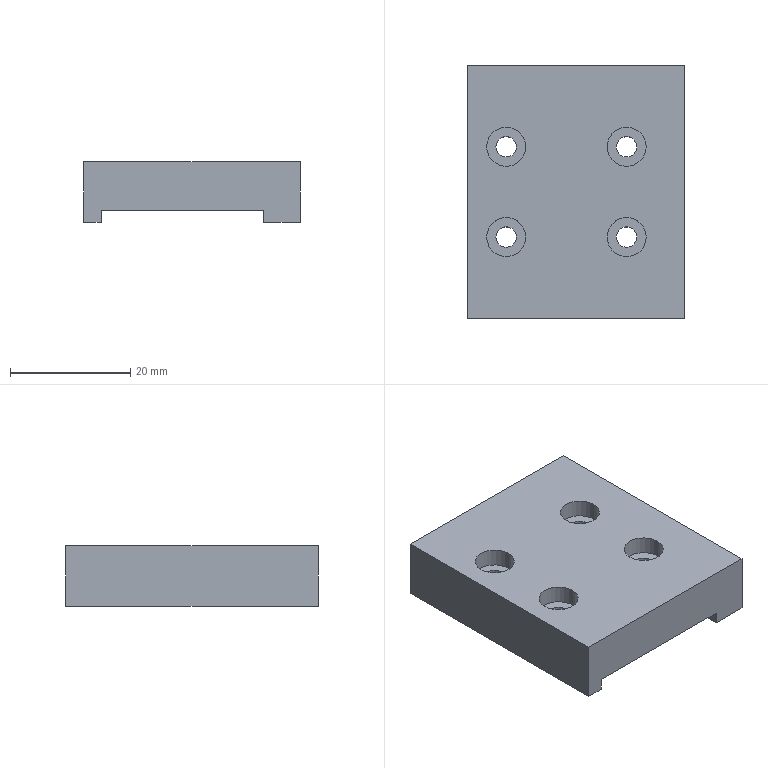Part | NX | features BREP 1 | 1 solid | 30 faces | box 36 x 42 x 10 mm | volume 12272 mm3 | cylinder 16 | plane 14 | commonest cylinder face diameters 3.4 x8 6.5 x8
STEP:
#1=CARTESIAN_POINT('',(-13.25,63.775,7.));
#2=VERTEX_POINT('',#1);
#3=CARTESIAN_POINT('',(-6.75,63.775,7.));
#4=VERTEX_POINT('',#3);
#5=CARTESIAN_POINT('',(-10.,63.775,7.));
#6=DIRECTION('',(0.,0.,1.));
#7=DIRECTION('',(1.,0.,0.));
#8=AXIS2_PLACEMENT_3D('',#5,#6,#7);
#9=CIRCLE('',#8,3.25);
#10=EDGE_CURVE('',#2,#4,#9,.T.);
#11=ORIENTED_EDGE('',*,*,#10,.F.);
#12=CARTESIAN_POINT('',(-13.25,63.775,10.));
#13=VERTEX_POINT('',#12);
#14=CARTESIAN_POINT('',(-13.25,63.775,10.));
#15=DIRECTION('',(0.,0.,1.));
#16=VECTOR('',#15,1000.);
#17=LINE('',#14,#16);
#18=EDGE_CURVE('',#13,#2,#17,.F.);
#19=ORIENTED_EDGE('',*,*,#18,.F.);
#20=CARTESIAN_POINT('',(-6.75,63.775,10.));
#21=VERTEX_POINT('',#20);
#22=CARTESIAN_POINT('',(-10.,63.775,10.));
#23=DIRECTION('',(0.,0.,1.));
#24=DIRECTION('',(1.,0.,0.));
#25=AXIS2_PLACEMENT_3D('',#22,#23,#24);
#26=CIRCLE('',#25,3.25);
#27=EDGE_CURVE('',#13,#21,#26,.T.);
#28=ORIENTED_EDGE('',*,*,#27,.T.);
#29=CARTESIAN_POINT('',(-6.75,63.775,10.));
#30=DIRECTION('',(0.,0.,1.));
#31=VECTOR('',#30,1000.);
#32=LINE('',#29,#31);
#33=EDGE_CURVE('',#21,#4,#32,.F.);
#34=ORIENTED_EDGE('',*,*,#33,.T.);
#35=EDGE_LOOP('',(#11,#19,#28,#34));
#36=FACE_BOUND('',#35,.T.);
#37=CARTESIAN_POINT('',(-10.,63.775,10.));
#38=DIRECTION('',(0.,0.,1.));
#39=DIRECTION('',(1.,0.,0.));
#40=AXIS2_PLACEMENT_3D('',#37,#38,#39);
#41=CYLINDRICAL_SURFACE('',#40,3.25);
#42=ADVANCED_FACE('',(#36),#41,.F.);
#43=CARTESIAN_POINT('',(-11.7,63.775,2.));
#44=VERTEX_POINT('',#43);
#45=CARTESIAN_POINT('',(-8.3,63.775,2.));
#46=VERTEX_POINT('',#45);
#47=CARTESIAN_POINT('',(-10.,63.775,2.));
#48=DIRECTION('',(0.,0.,1.));
#49=DIRECTION('',(1.,0.,0.));
#50=AXIS2_PLACEMENT_3D('',#47,#48,#49);
#51=CIRCLE('',#50,1.7);
#52=EDGE_CURVE('',#44,#46,#51,.T.);
#53=ORIENTED_EDGE('',*,*,#52,.F.);
#54=CARTESIAN_POINT('',(-11.7,63.775,7.));
#55=VERTEX_POINT('',#54);
#56=CARTESIAN_POINT('',(-11.7,63.775,10.));
#57=DIRECTION('',(0.,0.,1.));
#58=VECTOR('',#57,1000.);
#59=LINE('',#56,#58);
#60=EDGE_CURVE('',#55,#44,#59,.F.);
#61=ORIENTED_EDGE('',*,*,#60,.F.);
#62=CARTESIAN_POINT('',(-8.3,63.775,7.));
#63=VERTEX_POINT('',#62);
#64=CARTESIAN_POINT('',(-10.,63.775,7.));
#65=DIRECTION('',(0.,0.,1.));
#66=DIRECTION('',(1.,0.,0.));
#67=AXIS2_PLACEMENT_3D('',#64,#65,#66);
#68=CIRCLE('',#67,1.7);
#69=EDGE_CURVE('',#55,#63,#68,.T.);
#70=ORIENTED_EDGE('',*,*,#69,.T.);
#71=CARTESIAN_POINT('',(-8.3,63.775,10.));
#72=DIRECTION('',(0.,0.,1.));
#73=VECTOR('',#72,1000.);
#74=LINE('',#71,#73);
#75=EDGE_CURVE('',#63,#46,#74,.F.);
#76=ORIENTED_EDGE('',*,*,#75,.T.);
#77=EDGE_LOOP('',(#53,#61,#70,#76));
#78=FACE_BOUND('',#77,.T.);
#79=CARTESIAN_POINT('',(-10.,63.775,10.));
#80=DIRECTION('',(0.,0.,1.));
#81=DIRECTION('',(1.,0.,0.));
#82=AXIS2_PLACEMENT_3D('',#79,#80,#81);
#83=CYLINDRICAL_SURFACE('',#82,1.7);
#84=ADVANCED_FACE('',(#78),#83,.F.);
#85=CARTESIAN_POINT('',(-13.25,78.775,7.));
#86=VERTEX_POINT('',#85);
#87=CARTESIAN_POINT('',(-6.75,78.775,7.));
#88=VERTEX_POINT('',#87);
#89=CARTESIAN_POINT('',(-10.,78.775,7.));
#90=DIRECTION('',(0.,0.,1.));
#91=DIRECTION('',(1.,0.,0.));
#92=AXIS2_PLACEMENT_3D('',#89,#90,#91);
#93=CIRCLE('',#92,3.25);
#94=EDGE_CURVE('',#86,#88,#93,.T.);
#95=ORIENTED_EDGE('',*,*,#94,.F.);
#96=CARTESIAN_POINT('',(-13.25,78.775,10.));
#97=VERTEX_POINT('',#96);
#98=CARTESIAN_POINT('',(-13.25,78.775,10.));
#99=DIRECTION('',(0.,0.,1.));
#100=VECTOR('',#99,1000.);
#101=LINE('',#98,#100);
#102=EDGE_CURVE('',#97,#86,#101,.F.);
#103=ORIENTED_EDGE('',*,*,#102,.F.);
#104=CARTESIAN_POINT('',(-6.75,78.775,10.));
#105=VERTEX_POINT('',#104);
#106=CARTESIAN_POINT('',(-10.,78.775,10.));
#107=DIRECTION('',(0.,0.,1.));
#108=DIRECTION('',(1.,0.,0.));
#109=AXIS2_PLACEMENT_3D('',#106,#107,#108);
#110=CIRCLE('',#109,3.25);
#111=EDGE_CURVE('',#97,#105,#110,.T.);
#112=ORIENTED_EDGE('',*,*,#111,.T.);
#113=CARTESIAN_POINT('',(-6.75,78.775,10.));
#114=DIRECTION('',(0.,0.,1.));
#115=VECTOR('',#114,1000.);
#116=LINE('',#113,#115);
#117=EDGE_CURVE('',#105,#88,#116,.F.);
#118=ORIENTED_EDGE('',*,*,#117,.T.);
#119=EDGE_LOOP('',(#95,#103,#112,#118));
#120=FACE_BOUND('',#119,.T.);
#121=CARTESIAN_POINT('',(-10.,78.775,10.));
#122=DIRECTION('',(0.,0.,1.));
#123=DIRECTION('',(1.,0.,0.));
#124=AXIS2_PLACEMENT_3D('',#121,#122,#123);
#125=CYLINDRICAL_SURFACE('',#124,3.25);
#126=ADVANCED_FACE('',(#120),#125,.F.);
#127=CARTESIAN_POINT('',(-11.7,78.775,2.));
#128=VERTEX_POINT('',#127);
#129=CARTESIAN_POINT('',(-8.3,78.775,2.));
#130=VERTEX_POINT('',#129);
#131=CARTESIAN_POINT('',(-10.,78.775,2.));
#132=DIRECTION('',(0.,0.,1.));
#133=DIRECTION('',(1.,0.,0.));
#134=AXIS2_PLACEMENT_3D('',#131,#132,#133);
#135=CIRCLE('',#134,1.7);
#136=EDGE_CURVE('',#128,#130,#135,.T.);
#137=ORIENTED_EDGE('',*,*,#136,.F.);
#138=CARTESIAN_POINT('',(-11.7,78.775,7.));
#139=VERTEX_POINT('',#138);
#140=CARTESIAN_POINT('',(-11.7,78.775,10.));
#141=DIRECTION('',(0.,0.,1.));
#142=VECTOR('',#141,1000.);
#143=LINE('',#140,#142);
#144=EDGE_CURVE('',#139,#128,#143,.F.);
#145=ORIENTED_EDGE('',*,*,#144,.F.);
#146=CARTESIAN_POINT('',(-8.3,78.775,7.));
#147=VERTEX_POINT('',#146);
#148=CARTESIAN_POINT('',(-10.,78.775,7.));
#149=DIRECTION('',(0.,0.,1.));
#150=DIRECTION('',(1.,0.,0.));
#151=AXIS2_PLACEMENT_3D('',#148,#149,#150);
#152=CIRCLE('',#151,1.7);
#153=EDGE_CURVE('',#139,#147,#152,.T.);
#154=ORIENTED_EDGE('',*,*,#153,.T.);
#155=CARTESIAN_POINT('',(-8.3,78.775,10.));
#156=DIRECTION('',(0.,0.,1.));
#157=VECTOR('',#156,1000.);
#158=LINE('',#155,#157);
#159=EDGE_CURVE('',#147,#130,#158,.F.);
#160=ORIENTED_EDGE('',*,*,#159,.T.);
#161=EDGE_LOOP('',(#137,#145,#154,#160));
#162=FACE_BOUND('',#161,.T.);
#163=CARTESIAN_POINT('',(-10.,78.775,10.));
#164=DIRECTION('',(0.,0.,1.));
#165=DIRECTION('',(1.,0.,0.));
#166=AXIS2_PLACEMENT_3D('',#163,#164,#165);
#167=CYLINDRICAL_SURFACE('',#166,1.7);
#168=ADVANCED_FACE('',(#162),#167,.F.);
#169=CARTESIAN_POINT('',(6.75,63.775,7.));
#170=VERTEX_POINT('',#169);
#171=CARTESIAN_POINT('',(13.25,63.775,7.));
#172=VERTEX_POINT('',#171);
#173=CARTESIAN_POINT('',(10.,63.775,7.));
#174=DIRECTION('',(0.,0.,1.));
#175=DIRECTION('',(1.,0.,0.));
#176=AXIS2_PLACEMENT_3D('',#173,#174,#175);
#177=CIRCLE('',#176,3.25);
#178=EDGE_CURVE('',#170,#172,#177,.T.);
#179=ORIENTED_EDGE('',*,*,#178,.F.);
#180=CARTESIAN_POINT('',(6.75,63.775,10.));
#181=VERTEX_POINT('',#180);
#182=CARTESIAN_POINT('',(6.75,63.775,10.));
#183=DIRECTION('',(0.,0.,1.));
#184=VECTOR('',#183,1000.);
#185=LINE('',#182,#184);
#186=EDGE_CURVE('',#181,#170,#185,.F.);
#187=ORIENTED_EDGE('',*,*,#186,.F.);
#188=CARTESIAN_POINT('',(13.25,63.775,10.));
#189=VERTEX_POINT('',#188);
#190=CARTESIAN_POINT('',(10.,63.775,10.));
#191=DIRECTION('',(0.,0.,1.));
#192=DIRECTION('',(1.,0.,0.));
#193=AXIS2_PLACEMENT_3D('',#190,#191,#192);
#194=CIRCLE('',#193,3.25);
#195=EDGE_CURVE('',#181,#189,#194,.T.);
#196=ORIENTED_EDGE('',*,*,#195,.T.);
#197=CARTESIAN_POINT('',(13.25,63.775,10.));
#198=DIRECTION('',(0.,0.,1.));
#199=VECTOR('',#198,1000.);
#200=LINE('',#197,#199);
#201=EDGE_CURVE('',#189,#172,#200,.F.);
#202=ORIENTED_EDGE('',*,*,#201,.T.);
#203=EDGE_LOOP('',(#179,#187,#196,#202));
#204=FACE_BOUND('',#203,.T.);
#205=CARTESIAN_POINT('',(10.,63.775,10.));
#206=DIRECTION('',(0.,0.,1.));
#207=DIRECTION('',(1.,0.,0.));
#208=AXIS2_PLACEMENT_3D('',#205,#206,#207);
#209=CYLINDRICAL_SURFACE('',#208,3.25);
#210=ADVANCED_FACE('',(#204),#209,.F.);
#211=CARTESIAN_POINT('',(8.3,63.775,2.));
#212=VERTEX_POINT('',#211);
#213=CARTESIAN_POINT('',(11.7,63.775,2.));
#214=VERTEX_POINT('',#213);
#215=CARTESIAN_POINT('',(10.,63.775,2.));
#216=DIRECTION('',(0.,0.,1.));
#217=DIRECTION('',(1.,0.,0.));
#218=AXIS2_PLACEMENT_3D('',#215,#216,#217);
#219=CIRCLE('',#218,1.7);
#220=EDGE_CURVE('',#212,#214,#219,.T.);
#221=ORIENTED_EDGE('',*,*,#220,.F.);
#222=CARTESIAN_POINT('',(8.3,63.775,7.));
#223=VERTEX_POINT('',#222);
#224=CARTESIAN_POINT('',(8.3,63.775,10.));
#225=DIRECTION('',(0.,0.,1.));
#226=VECTOR('',#225,1000.);
#227=LINE('',#224,#226);
#228=EDGE_CURVE('',#223,#212,#227,.F.);
#229=ORIENTED_EDGE('',*,*,#228,.F.);
#230=CARTESIAN_POINT('',(11.7,63.775,7.));
#231=VERTEX_POINT('',#230);
#232=CARTESIAN_POINT('',(10.,63.775,7.));
#233=DIRECTION('',(0.,0.,1.));
#234=DIRECTION('',(1.,0.,0.));
#235=AXIS2_PLACEMENT_3D('',#232,#233,#234);
#236=CIRCLE('',#235,1.7);
#237=EDGE_CURVE('',#223,#231,#236,.T.);
#238=ORIENTED_EDGE('',*,*,#237,.T.);
#239=CARTESIAN_POINT('',(11.7,63.775,10.));
#240=DIRECTION('',(0.,0.,1.));
#241=VECTOR('',#240,1000.);
#242=LINE('',#239,#241);
#243=EDGE_CURVE('',#231,#214,#242,.F.);
#244=ORIENTED_EDGE('',*,*,#243,.T.);
#245=EDGE_LOOP('',(#221,#229,#238,#244));
#246=FACE_BOUND('',#245,.T.);
#247=CARTESIAN_POINT('',(10.,63.775,10.));
#248=DIRECTION('',(0.,0.,1.));
#249=DIRECTION('',(1.,0.,0.));
#250=AXIS2_PLACEMENT_3D('',#247,#248,#249);
#251=CYLINDRICAL_SURFACE('',#250,1.7);
#252=ADVANCED_FACE('',(#246),#251,.F.);
#253=CARTESIAN_POINT('',(6.75,78.775,7.));
#254=VERTEX_POINT('',#253);
#255=CARTESIAN_POINT('',(13.25,78.775,7.));
#256=VERTEX_POINT('',#255);
#257=CARTESIAN_POINT('',(10.,78.775,7.));
#258=DIRECTION('',(0.,0.,1.));
#259=DIRECTION('',(1.,0.,0.));
#260=AXIS2_PLACEMENT_3D('',#257,#258,#259);
#261=CIRCLE('',#260,3.25);
#262=EDGE_CURVE('',#254,#256,#261,.T.);
#263=ORIENTED_EDGE('',*,*,#262,.F.);
#264=CARTESIAN_POINT('',(6.75,78.775,10.));
#265=VERTEX_POINT('',#264);
#266=CARTESIAN_POINT('',(6.75,78.775,10.));
#267=DIRECTION('',(0.,0.,1.));
#268=VECTOR('',#267,1000.);
#269=LINE('',#266,#268);
#270=EDGE_CURVE('',#265,#254,#269,.F.);
#271=ORIENTED_EDGE('',*,*,#270,.F.);
#272=CARTESIAN_POINT('',(13.25,78.775,10.));
#273=VERTEX_POINT('',#272);
#274=CARTESIAN_POINT('',(10.,78.775,10.));
#275=DIRECTION('',(0.,0.,1.));
#276=DIRECTION('',(1.,0.,0.));
#277=AXIS2_PLACEMENT_3D('',#274,#275,#276);
#278=CIRCLE('',#277,3.25);
#279=EDGE_CURVE('',#265,#273,#278,.T.);
#280=ORIENTED_EDGE('',*,*,#279,.T.);
#281=CARTESIAN_POINT('',(13.25,78.775,10.));
#282=DIRECTION('',(0.,0.,1.));
#283=VECTOR('',#282,1000.);
#284=LINE('',#281,#283);
#285=EDGE_CURVE('',#273,#256,#284,.F.);
#286=ORIENTED_EDGE('',*,*,#285,.T.);
#287=EDGE_LOOP('',(#263,#271,#280,#286));
#288=FACE_BOUND('',#287,.T.);
#289=CARTESIAN_POINT('',(10.,78.775,10.));
#290=DIRECTION('',(0.,0.,1.));
#291=DIRECTION('',(1.,0.,0.));
#292=AXIS2_PLACEMENT_3D('',#289,#290,#291);
#293=CYLINDRICAL_SURFACE('',#292,3.25);
#294=ADVANCED_FACE('',(#288),#293,.F.);
#295=CARTESIAN_POINT('',(8.3,78.775,2.));
#296=VERTEX_POINT('',#295);
#297=CARTESIAN_POINT('',(11.7,78.775,2.));
#298=VERTEX_POINT('',#297);
#299=CARTESIAN_POINT('',(10.,78.775,2.));
#300=DIRECTION('',(0.,0.,1.));
#301=DIRECTION('',(1.,0.,0.));
#302=AXIS2_PLACEMENT_3D('',#299,#300,#301);
#303=CIRCLE('',#302,1.7);
#304=EDGE_CURVE('',#296,#298,#303,.T.);
#305=ORIENTED_EDGE('',*,*,#304,.F.);
#306=CARTESIAN_POINT('',(8.3,78.775,7.));
#307=VERTEX_POINT('',#306);
#308=CARTESIAN_POINT('',(8.3,78.775,10.));
#309=DIRECTION('',(0.,0.,1.));
#310=VECTOR('',#309,1000.);
#311=LINE('',#308,#310);
#312=EDGE_CURVE('',#307,#296,#311,.F.);
#313=ORIENTED_EDGE('',*,*,#312,.F.);
#314=CARTESIAN_POINT('',(11.7,78.775,7.));
#315=VERTEX_POINT('',#314);
#316=CARTESIAN_POINT('',(10.,78.775,7.));
#317=DIRECTION('',(0.,0.,1.));
#318=DIRECTION('',(1.,0.,0.));
#319=AXIS2_PLACEMENT_3D('',#316,#317,#318);
#320=CIRCLE('',#319,1.7);
#321=EDGE_CURVE('',#307,#315,#320,.T.);
#322=ORIENTED_EDGE('',*,*,#321,.T.);
#323=CARTESIAN_POINT('',(11.7,78.775,10.));
#324=DIRECTION('',(0.,0.,1.));
#325=VECTOR('',#324,1000.);
#326=LINE('',#323,#325);
#327=EDGE_CURVE('',#315,#298,#326,.F.);
#328=ORIENTED_EDGE('',*,*,#327,.T.);
#329=EDGE_LOOP('',(#305,#313,#322,#328));
#330=FACE_BOUND('',#329,.T.);
#331=CARTESIAN_POINT('',(10.,78.775,10.));
#332=DIRECTION('',(0.,0.,1.));
#333=DIRECTION('',(1.,0.,0.));
#334=AXIS2_PLACEMENT_3D('',#331,#332,#333);
#335=CYLINDRICAL_SURFACE('',#334,1.7);
#336=ADVANCED_FACE('',(#330),#335,.F.);
#337=CARTESIAN_POINT('',(-13.5,92.275,0.));
#338=VERTEX_POINT('',#337);
#339=CARTESIAN_POINT('',(-16.407,92.275,0.));
#340=VERTEX_POINT('',#339);
#341=CARTESIAN_POINT('',(-16.407,92.275,0.));
#342=DIRECTION('',(-1.,0.,0.));
#343=VECTOR('',#342,1000.);
#344=LINE('',#341,#343);
#345=EDGE_CURVE('',#338,#340,#344,.T.);
#346=ORIENTED_EDGE('',*,*,#345,.F.);
#347=CARTESIAN_POINT('',(-13.5,50.275,0.));
#348=VERTEX_POINT('',#347);
#349=CARTESIAN_POINT('',(-13.5,92.275,0.));
#350=DIRECTION('',(0.,-1.,0.));
#351=VECTOR('',#350,1000.);
#352=LINE('',#349,#351);
#353=EDGE_CURVE('',#338,#348,#352,.T.);
#354=ORIENTED_EDGE('',*,*,#353,.T.);
#355=CARTESIAN_POINT('',(-16.407,50.275,0.));
#356=VERTEX_POINT('',#355);
#357=CARTESIAN_POINT('',(-16.407,50.275,0.));
#358=DIRECTION('',(1.,0.,0.));
#359=VECTOR('',#358,1000.);
#360=LINE('',#357,#359);
#361=EDGE_CURVE('',#356,#348,#360,.T.);
#362=ORIENTED_EDGE('',*,*,#361,.F.);
#363=CARTESIAN_POINT('',(-16.407,92.275,0.));
#364=DIRECTION('',(0.,-1.,0.));
#365=VECTOR('',#364,1000.);
#366=LINE('',#363,#365);
#367=EDGE_CURVE('',#340,#356,#366,.T.);
#368=ORIENTED_EDGE('',*,*,#367,.F.);
#369=EDGE_LOOP('',(#346,#354,#362,#368));
#370=FACE_BOUND('',#369,.T.);
#371=CARTESIAN_POINT('',(-16.407,50.275,0.));
#372=DIRECTION('',(0.,0.,1.));
#373=DIRECTION('',(1.,0.,0.));
#374=AXIS2_PLACEMENT_3D('',#371,#372,#373);
#375=PLANE('',#374);
#376=ADVANCED_FACE('',(#370),#375,.F.);
#377=ORIENTED_EDGE('',*,*,#367,.T.);
#378=CARTESIAN_POINT('',(-16.407,50.275,10.));
#379=VERTEX_POINT('',#378);
#380=CARTESIAN_POINT('',(-16.407,50.275,10.));
#381=DIRECTION('',(0.,0.,-1.));
#382=VECTOR('',#381,1000.);
#383=LINE('',#380,#382);
#384=EDGE_CURVE('',#379,#356,#383,.T.);
#385=ORIENTED_EDGE('',*,*,#384,.F.);
#386=CARTESIAN_POINT('',(-16.407,92.275,10.));
#387=VERTEX_POINT('',#386);
#388=CARTESIAN_POINT('',(-16.407,92.275,10.));
#389=DIRECTION('',(0.,-1.,0.));
#390=VECTOR('',#389,1000.);
#391=LINE('',#388,#390);
#392=EDGE_CURVE('',#387,#379,#391,.T.);
#393=ORIENTED_EDGE('',*,*,#392,.F.);
#394=CARTESIAN_POINT('',(-16.407,92.275,10.));
#395=DIRECTION('',(0.,0.,-1.));
#396=VECTOR('',#395,1000.);
#397=LINE('',#394,#396);
#398=EDGE_CURVE('',#387,#340,#397,.T.);
#399=ORIENTED_EDGE('',*,*,#398,.T.);
#400=EDGE_LOOP('',(#377,#385,#393,#399));
#401=FACE_BOUND('',#400,.T.);
#402=CARTESIAN_POINT('',(-16.407,92.275,10.));
#403=DIRECTION('',(1.,0.,0.));
#404=DIRECTION('',(0.,1.,0.));
#405=AXIS2_PLACEMENT_3D('',#402,#403,#404);
#406=PLANE('',#405);
#407=ADVANCED_FACE('',(#401),#406,.F.);
#408=ORIENTED_EDGE('',*,*,#361,.T.);
#409=CARTESIAN_POINT('',(-13.5,50.275,2.));
#410=VERTEX_POINT('',#409);
#411=CARTESIAN_POINT('',(-13.5,50.275,0.));
#412=DIRECTION('',(0.,0.,-1.));
#413=VECTOR('',#412,1000.);
#414=LINE('',#411,#413);
#415=EDGE_CURVE('',#410,#348,#414,.T.);
#416=ORIENTED_EDGE('',*,*,#415,.F.);
#417=CARTESIAN_POINT('',(13.5,50.275,2.));
#418=VERTEX_POINT('',#417);
#419=CARTESIAN_POINT('',(-13.5,50.275,2.));
#420=DIRECTION('',(-1.,0.,0.));
#421=VECTOR('',#420,1000.);
#422=LINE('',#419,#421);
#423=EDGE_CURVE('',#418,#410,#422,.T.);
#424=ORIENTED_EDGE('',*,*,#423,.F.);
#425=CARTESIAN_POINT('',(13.5,50.275,0.));
#426=VERTEX_POINT('',#425);
#427=CARTESIAN_POINT('',(13.5,50.275,0.));
#428=DIRECTION('',(0.,0.,1.));
#429=VECTOR('',#428,1000.);
#430=LINE('',#427,#429);
#431=EDGE_CURVE('',#426,#418,#430,.T.);
#432=ORIENTED_EDGE('',*,*,#431,.F.);
#433=CARTESIAN_POINT('',(19.593,50.275,0.));
#434=VERTEX_POINT('',#433);
#435=CARTESIAN_POINT('',(-16.407,50.275,0.));
#436=DIRECTION('',(1.,0.,0.));
#437=VECTOR('',#436,1000.);
#438=LINE('',#435,#437);
#439=EDGE_CURVE('',#426,#434,#438,.T.);
#440=ORIENTED_EDGE('',*,*,#439,.T.);
#441=CARTESIAN_POINT('',(19.593,50.275,10.));
#442=VERTEX_POINT('',#441);
#443=CARTESIAN_POINT('',(19.593,50.275,10.));
#444=DIRECTION('',(0.,0.,-1.));
#445=VECTOR('',#444,1000.);
#446=LINE('',#443,#445);
#447=EDGE_CURVE('',#442,#434,#446,.T.);
#448=ORIENTED_EDGE('',*,*,#447,.F.);
#449=CARTESIAN_POINT('',(-16.407,50.275,10.));
#450=DIRECTION('',(1.,0.,0.));
#451=VECTOR('',#450,1000.);
#452=LINE('',#449,#451);
#453=EDGE_CURVE('',#379,#442,#452,.T.);
#454=ORIENTED_EDGE('',*,*,#453,.F.);
#455=ORIENTED_EDGE('',*,*,#384,.T.);
#456=EDGE_LOOP('',(#408,#416,#424,#432,#440,#448,#454,#455));
#457=FACE_BOUND('',#456,.T.);
#458=CARTESIAN_POINT('',(-16.407,50.275,10.));
#459=DIRECTION('',(0.,1.,0.));
#460=DIRECTION('',(1.,0.,0.));
#461=AXIS2_PLACEMENT_3D('',#458,#459,#460);
#462=PLANE('',#461);
#463=ADVANCED_FACE('',(#457),#462,.F.);
#464=CARTESIAN_POINT('',(19.593,92.275,0.));
#465=VERTEX_POINT('',#464);
#466=CARTESIAN_POINT('',(19.593,92.275,0.));
#467=DIRECTION('',(0.,1.,0.));
#468=VECTOR('',#467,1000.);
#469=LINE('',#466,#468);
#470=EDGE_CURVE('',#434,#465,#469,.T.);
#471=ORIENTED_EDGE('',*,*,#470,.T.);
#472=CARTESIAN_POINT('',(19.593,92.275,10.));
#473=VERTEX_POINT('',#472);
#474=CARTESIAN_POINT('',(19.593,92.275,10.));
#475=DIRECTION('',(0.,0.,-1.));
#476=VECTOR('',#475,1000.);
#477=LINE('',#474,#476);
#478=EDGE_CURVE('',#473,#465,#477,.T.);
#479=ORIENTED_EDGE('',*,*,#478,.F.);
#480=CARTESIAN_POINT('',(19.593,92.275,10.));
#481=DIRECTION('',(0.,1.,0.));
#482=VECTOR('',#481,1000.);
#483=LINE('',#480,#482);
#484=EDGE_CURVE('',#442,#473,#483,.T.);
#485=ORIENTED_EDGE('',*,*,#484,.F.);
#486=ORIENTED_EDGE('',*,*,#447,.T.);
#487=EDGE_LOOP('',(#471,#479,#485,#486));
#488=FACE_BOUND('',#487,.T.);
#489=CARTESIAN_POINT('',(19.593,92.275,10.));
#490=DIRECTION('',(-1.,0.,0.));
#491=DIRECTION('',(0.,0.,1.));
#492=AXIS2_PLACEMENT_3D('',#489,#490,#491);
#493=PLANE('',#492);
#494=ADVANCED_FACE('',(#488),#493,.F.);
#495=CARTESIAN_POINT('',(13.5,92.275,2.));
#496=VERTEX_POINT('',#495);
#497=CARTESIAN_POINT('',(-13.5,92.275,2.));
#498=VERTEX_POINT('',#497);
#499=CARTESIAN_POINT('',(-13.5,92.275,2.));
#500=DIRECTION('',(-1.,0.,0.));
#501=VECTOR('',#500,1000.);
#502=LINE('',#499,#501);
#503=EDGE_CURVE('',#496,#498,#502,.T.);
#504=ORIENTED_EDGE('',*,*,#503,.T.);
#505=CARTESIAN_POINT('',(-13.5,92.275,0.));
#506=DIRECTION('',(0.,0.,-1.));
#507=VECTOR('',#506,1000.);
#508=LINE('',#505,#507);
#509=EDGE_CURVE('',#498,#338,#508,.T.);
#510=ORIENTED_EDGE('',*,*,#509,.T.);
#511=ORIENTED_EDGE('',*,*,#345,.T.);
#512=ORIENTED_EDGE('',*,*,#398,.F.);
#513=CARTESIAN_POINT('',(-16.407,92.275,10.));
#514=DIRECTION('',(-1.,0.,0.));
#515=VECTOR('',#514,1000.);
#516=LINE('',#513,#515);
#517=EDGE_CURVE('',#473,#387,#516,.T.);
#518=ORIENTED_EDGE('',*,*,#517,.F.);
#519=ORIENTED_EDGE('',*,*,#478,.T.);
#520=CARTESIAN_POINT('',(13.5,92.275,0.));
#521=VERTEX_POINT('',#520);
#522=CARTESIAN_POINT('',(-16.407,92.275,0.));
#523=DIRECTION('',(-1.,0.,0.));
#524=VECTOR('',#523,1000.);
#525=LINE('',#522,#524);
#526=EDGE_CURVE('',#465,#521,#525,.T.);
#527=ORIENTED_EDGE('',*,*,#526,.T.);
#528=CARTESIAN_POINT('',(13.5,92.275,0.));
#529=DIRECTION('',(0.,0.,1.));
#530=VECTOR('',#529,1000.);
#531=LINE('',#528,#530);
#532=EDGE_CURVE('',#521,#496,#531,.T.);
#533=ORIENTED_EDGE('',*,*,#532,.T.);
#534=EDGE_LOOP('',(#504,#510,#511,#512,#518,#519,#527,#533));
#535=FACE_BOUND('',#534,.T.);
#536=CARTESIAN_POINT('',(-16.407,92.275,10.));
#537=DIRECTION('',(0.,-1.,0.));
#538=DIRECTION('',(0.,0.,-1.));
#539=AXIS2_PLACEMENT_3D('',#536,#537,#538);
#540=PLANE('',#539);
#541=ADVANCED_FACE('',(#535),#540,.F.);
#542=ORIENTED_EDGE('',*,*,#392,.T.);
#543=ORIENTED_EDGE('',*,*,#453,.T.);
#544=ORIENTED_EDGE('',*,*,#484,.T.);
#545=ORIENTED_EDGE('',*,*,#517,.T.);
#546=EDGE_LOOP('',(#542,#543,#544,#545));
#547=FACE_BOUND('',#546,.T.);
#548=CARTESIAN_POINT('',(-10.,63.775,10.));
#549=DIRECTION('',(0.,0.,1.));
#550=DIRECTION('',(1.,0.,0.));
#551=AXIS2_PLACEMENT_3D('',#548,#549,#550);
#552=CIRCLE('',#551,3.25);
#553=EDGE_CURVE('',#21,#13,#552,.T.);
#554=ORIENTED_EDGE('',*,*,#553,.F.);
#555=ORIENTED_EDGE('',*,*,#27,.F.);
#556=EDGE_LOOP('',(#554,#555));
#557=FACE_BOUND('',#556,.T.);
#558=CARTESIAN_POINT('',(-10.,78.775,10.));
#559=DIRECTION('',(0.,0.,1.));
#560=DIRECTION('',(1.,0.,0.));
#561=AXIS2_PLACEMENT_3D('',#558,#559,#560);
#562=CIRCLE('',#561,3.25);
#563=EDGE_CURVE('',#105,#97,#562,.T.);
#564=ORIENTED_EDGE('',*,*,#563,.F.);
#565=ORIENTED_EDGE('',*,*,#111,.F.);
#566=EDGE_LOOP('',(#564,#565));
#567=FACE_BOUND('',#566,.T.);
#568=CARTESIAN_POINT('',(10.,63.775,10.));
#569=DIRECTION('',(0.,0.,1.));
#570=DIRECTION('',(1.,0.,0.));
#571=AXIS2_PLACEMENT_3D('',#568,#569,#570);
#572=CIRCLE('',#571,3.25);
#573=EDGE_CURVE('',#189,#181,#572,.T.);
#574=ORIENTED_EDGE('',*,*,#573,.F.);
#575=ORIENTED_EDGE('',*,*,#195,.F.);
#576=EDGE_LOOP('',(#574,#575));
#577=FACE_BOUND('',#576,.T.);
#578=CARTESIAN_POINT('',(10.,78.775,10.));
#579=DIRECTION('',(0.,0.,1.));
#580=DIRECTION('',(1.,0.,0.));
#581=AXIS2_PLACEMENT_3D('',#578,#579,#580);
#582=CIRCLE('',#581,3.25);
#583=EDGE_CURVE('',#273,#265,#582,.T.);
#584=ORIENTED_EDGE('',*,*,#583,.F.);
#585=ORIENTED_EDGE('',*,*,#279,.F.);
#586=EDGE_LOOP('',(#584,#585));
#587=FACE_BOUND('',#586,.T.);
#588=CARTESIAN_POINT('',(-16.407,50.275,10.));
#589=DIRECTION('',(0.,0.,1.));
#590=DIRECTION('',(1.,0.,0.));
#591=AXIS2_PLACEMENT_3D('',#588,#589,#590);
#592=PLANE('',#591);
#593=ADVANCED_FACE('',(#547,#557,#567,#577,#587),#592,.T.);
#594=ORIENTED_EDGE('',*,*,#439,.F.);
#595=CARTESIAN_POINT('',(13.5,92.275,0.));
#596=DIRECTION('',(0.,-1.,0.));
#597=VECTOR('',#596,1000.);
#598=LINE('',#595,#597);
#599=EDGE_CURVE('',#521,#426,#598,.T.);
#600=ORIENTED_EDGE('',*,*,#599,.F.);
#601=ORIENTED_EDGE('',*,*,#526,.F.);
#602=ORIENTED_EDGE('',*,*,#470,.F.);
#603=EDGE_LOOP('',(#594,#600,#601,#602));
#604=FACE_BOUND('',#603,.T.);
#605=CARTESIAN_POINT('',(-16.407,50.275,0.));
#606=DIRECTION('',(0.,0.,1.));
#607=DIRECTION('',(1.,0.,0.));
#608=AXIS2_PLACEMENT_3D('',#605,#606,#607);
#609=PLANE('',#608);
#610=ADVANCED_FACE('',(#604),#609,.F.);
#611=ORIENTED_EDGE('',*,*,#415,.T.);
#612=ORIENTED_EDGE('',*,*,#353,.F.);
#613=ORIENTED_EDGE('',*,*,#509,.F.);
#614=CARTESIAN_POINT('',(-13.5,92.275,2.));
#615=DIRECTION('',(0.,-1.,0.));
#616=VECTOR('',#615,1000.);
#617=LINE('',#614,#616);
#618=EDGE_CURVE('',#498,#410,#617,.T.);
#619=ORIENTED_EDGE('',*,*,#618,.T.);
#620=EDGE_LOOP('',(#611,#612,#613,#619));
#621=FACE_BOUND('',#620,.T.);
#622=CARTESIAN_POINT('',(-13.5,92.275,0.));
#623=DIRECTION('',(-1.,0.,0.));
#624=DIRECTION('',(0.,0.,1.));
#625=AXIS2_PLACEMENT_3D('',#622,#623,#624);
#626=PLANE('',#625);
#627=ADVANCED_FACE('',(#621),#626,.F.);
#628=ORIENTED_EDGE('',*,*,#423,.T.);
#629=ORIENTED_EDGE('',*,*,#618,.F.);
#630=ORIENTED_EDGE('',*,*,#503,.F.);
#631=CARTESIAN_POINT('',(13.5,92.275,2.));
#632=DIRECTION('',(0.,-1.,0.));
#633=VECTOR('',#632,1000.);
#634=LINE('',#631,#633);
#635=EDGE_CURVE('',#496,#418,#634,.T.);
#636=ORIENTED_EDGE('',*,*,#635,.T.);
#637=EDGE_LOOP('',(#628,#629,#630,#636));
#638=FACE_BOUND('',#637,.T.);
#639=CARTESIAN_POINT('',(-10.,63.775,2.));
#640=DIRECTION('',(0.,0.,1.));
#641=DIRECTION('',(1.,0.,0.));
#642=AXIS2_PLACEMENT_3D('',#639,#640,#641);
#643=CIRCLE('',#642,1.7);
#644=EDGE_CURVE('',#46,#44,#643,.T.);
#645=ORIENTED_EDGE('',*,*,#644,.T.);
#646=ORIENTED_EDGE('',*,*,#52,.T.);
#647=EDGE_LOOP('',(#645,#646));
#648=FACE_BOUND('',#647,.T.);
#649=CARTESIAN_POINT('',(-10.,78.775,2.));
#650=DIRECTION('',(0.,0.,1.));
#651=DIRECTION('',(1.,0.,0.));
#652=AXIS2_PLACEMENT_3D('',#649,#650,#651);
#653=CIRCLE('',#652,1.7);
#654=EDGE_CURVE('',#130,#128,#653,.T.);
#655=ORIENTED_EDGE('',*,*,#654,.T.);
#656=ORIENTED_EDGE('',*,*,#136,.T.);
#657=EDGE_LOOP('',(#655,#656));
#658=FACE_BOUND('',#657,.T.);
#659=CARTESIAN_POINT('',(10.,63.775,2.));
#660=DIRECTION('',(0.,0.,1.));
#661=DIRECTION('',(1.,0.,0.));
#662=AXIS2_PLACEMENT_3D('',#659,#660,#661);
#663=CIRCLE('',#662,1.7);
#664=EDGE_CURVE('',#214,#212,#663,.T.);
#665=ORIENTED_EDGE('',*,*,#664,.T.);
#666=ORIENTED_EDGE('',*,*,#220,.T.);
#667=EDGE_LOOP('',(#665,#666));
#668=FACE_BOUND('',#667,.T.);
#669=CARTESIAN_POINT('',(10.,78.775,2.));
#670=DIRECTION('',(0.,0.,1.));
#671=DIRECTION('',(1.,0.,0.));
#672=AXIS2_PLACEMENT_3D('',#669,#670,#671);
#673=CIRCLE('',#672,1.7);
#674=EDGE_CURVE('',#298,#296,#673,.T.);
#675=ORIENTED_EDGE('',*,*,#674,.T.);
#676=ORIENTED_EDGE('',*,*,#304,.T.);
#677=EDGE_LOOP('',(#675,#676));
#678=FACE_BOUND('',#677,.T.);
#679=CARTESIAN_POINT('',(-13.5,92.275,2.));
#680=DIRECTION('',(0.,0.,1.));
#681=DIRECTION('',(1.,0.,0.));
#682=AXIS2_PLACEMENT_3D('',#679,#680,#681);
#683=PLANE('',#682);
#684=ADVANCED_FACE('',(#638,#648,#658,#668,#678),#683,.F.);
#685=ORIENTED_EDGE('',*,*,#431,.T.);
#686=ORIENTED_EDGE('',*,*,#635,.F.);
#687=ORIENTED_EDGE('',*,*,#532,.F.);
#688=ORIENTED_EDGE('',*,*,#599,.T.);
#689=EDGE_LOOP('',(#685,#686,#687,#688));
#690=FACE_BOUND('',#689,.T.);
#691=CARTESIAN_POINT('',(13.5,92.275,0.));
#692=DIRECTION('',(1.,0.,0.));
#693=DIRECTION('',(0.,1.,0.));
#694=AXIS2_PLACEMENT_3D('',#691,#692,#693);
#695=PLANE('',#694);
#696=ADVANCED_FACE('',(#690),#695,.F.);
#697=ORIENTED_EDGE('',*,*,#312,.T.);
#698=ORIENTED_EDGE('',*,*,#674,.F.);
#699=ORIENTED_EDGE('',*,*,#327,.F.);
#700=CARTESIAN_POINT('',(10.,78.775,7.));
#701=DIRECTION('',(0.,0.,1.));
#702=DIRECTION('',(1.,0.,0.));
#703=AXIS2_PLACEMENT_3D('',#700,#701,#702);
#704=CIRCLE('',#703,1.7);
#705=EDGE_CURVE('',#315,#307,#704,.T.);
#706=ORIENTED_EDGE('',*,*,#705,.T.);
#707=EDGE_LOOP('',(#697,#698,#699,#706));
#708=FACE_BOUND('',#707,.T.);
#709=CARTESIAN_POINT('',(10.,78.775,10.));
#710=DIRECTION('',(0.,0.,1.));
#711=DIRECTION('',(1.,0.,0.));
#712=AXIS2_PLACEMENT_3D('',#709,#710,#711);
#713=CYLINDRICAL_SURFACE('',#712,1.7);
#714=ADVANCED_FACE('',(#708),#713,.F.);
#715=CARTESIAN_POINT('',(10.,78.775,7.));
#716=DIRECTION('',(0.,0.,1.));
#717=DIRECTION('',(1.,0.,0.));
#718=AXIS2_PLACEMENT_3D('',#715,#716,#717);
#719=CIRCLE('',#718,3.25);
#720=EDGE_CURVE('',#256,#254,#719,.T.);
#721=ORIENTED_EDGE('',*,*,#720,.T.);
#722=ORIENTED_EDGE('',*,*,#262,.T.);
#723=EDGE_LOOP('',(#721,#722));
#724=FACE_BOUND('',#723,.T.);
#725=ORIENTED_EDGE('',*,*,#705,.F.);
#726=ORIENTED_EDGE('',*,*,#321,.F.);
#727=EDGE_LOOP('',(#725,#726));
#728=FACE_BOUND('',#727,.T.);
#729=CARTESIAN_POINT('',(11.7,78.775,7.));
#730=DIRECTION('',(0.,0.,-1.));
#731=DIRECTION('',(0.,-1.,0.));
#732=AXIS2_PLACEMENT_3D('',#729,#730,#731);
#733=PLANE('',#732);
#734=ADVANCED_FACE('',(#724,#728),#733,.F.);
#735=ORIENTED_EDGE('',*,*,#270,.T.);
#736=ORIENTED_EDGE('',*,*,#720,.F.);
#737=ORIENTED_EDGE('',*,*,#285,.F.);
#738=ORIENTED_EDGE('',*,*,#583,.T.);
#739=EDGE_LOOP('',(#735,#736,#737,#738));
#740=FACE_BOUND('',#739,.T.);
#741=CARTESIAN_POINT('',(10.,78.775,10.));
#742=DIRECTION('',(0.,0.,1.));
#743=DIRECTION('',(1.,0.,0.));
#744=AXIS2_PLACEMENT_3D('',#741,#742,#743);
#745=CYLINDRICAL_SURFACE('',#744,3.25);
#746=ADVANCED_FACE('',(#740),#745,.F.);
#747=ORIENTED_EDGE('',*,*,#228,.T.);
#748=ORIENTED_EDGE('',*,*,#664,.F.);
#749=ORIENTED_EDGE('',*,*,#243,.F.);
#750=CARTESIAN_POINT('',(10.,63.775,7.));
#751=DIRECTION('',(0.,0.,1.));
#752=DIRECTION('',(1.,0.,0.));
#753=AXIS2_PLACEMENT_3D('',#750,#751,#752);
#754=CIRCLE('',#753,1.7);
#755=EDGE_CURVE('',#231,#223,#754,.T.);
#756=ORIENTED_EDGE('',*,*,#755,.T.);
#757=EDGE_LOOP('',(#747,#748,#749,#756));
#758=FACE_BOUND('',#757,.T.);
#759=CARTESIAN_POINT('',(10.,63.775,10.));
#760=DIRECTION('',(0.,0.,1.));
#761=DIRECTION('',(1.,0.,0.));
#762=AXIS2_PLACEMENT_3D('',#759,#760,#761);
#763=CYLINDRICAL_SURFACE('',#762,1.7);
#764=ADVANCED_FACE('',(#758),#763,.F.);
#765=CARTESIAN_POINT('',(10.,63.775,7.));
#766=DIRECTION('',(0.,0.,1.));
#767=DIRECTION('',(1.,0.,0.));
#768=AXIS2_PLACEMENT_3D('',#765,#766,#767);
#769=CIRCLE('',#768,3.25);
#770=EDGE_CURVE('',#172,#170,#769,.T.);
#771=ORIENTED_EDGE('',*,*,#770,.T.);
#772=ORIENTED_EDGE('',*,*,#178,.T.);
#773=EDGE_LOOP('',(#771,#772));
#774=FACE_BOUND('',#773,.T.);
#775=ORIENTED_EDGE('',*,*,#755,.F.);
#776=ORIENTED_EDGE('',*,*,#237,.F.);
#777=EDGE_LOOP('',(#775,#776));
#778=FACE_BOUND('',#777,.T.);
#779=CARTESIAN_POINT('',(11.7,63.775,7.));
#780=DIRECTION('',(0.,0.,-1.));
#781=DIRECTION('',(0.,-1.,0.));
#782=AXIS2_PLACEMENT_3D('',#779,#780,#781);
#783=PLANE('',#782);
#784=ADVANCED_FACE('',(#774,#778),#783,.F.);
#785=ORIENTED_EDGE('',*,*,#186,.T.);
#786=ORIENTED_EDGE('',*,*,#770,.F.);
#787=ORIENTED_EDGE('',*,*,#201,.F.);
#788=ORIENTED_EDGE('',*,*,#573,.T.);
#789=EDGE_LOOP('',(#785,#786,#787,#788));
#790=FACE_BOUND('',#789,.T.);
#791=CARTESIAN_POINT('',(10.,63.775,10.));
#792=DIRECTION('',(0.,0.,1.));
#793=DIRECTION('',(1.,0.,0.));
#794=AXIS2_PLACEMENT_3D('',#791,#792,#793);
#795=CYLINDRICAL_SURFACE('',#794,3.25);
#796=ADVANCED_FACE('',(#790),#795,.F.);
#797=ORIENTED_EDGE('',*,*,#144,.T.);
#798=ORIENTED_EDGE('',*,*,#654,.F.);
#799=ORIENTED_EDGE('',*,*,#159,.F.);
#800=CARTESIAN_POINT('',(-10.,78.775,7.));
#801=DIRECTION('',(0.,0.,1.));
#802=DIRECTION('',(1.,0.,0.));
#803=AXIS2_PLACEMENT_3D('',#800,#801,#802);
#804=CIRCLE('',#803,1.7);
#805=EDGE_CURVE('',#147,#139,#804,.T.);
#806=ORIENTED_EDGE('',*,*,#805,.T.);
#807=EDGE_LOOP('',(#797,#798,#799,#806));
#808=FACE_BOUND('',#807,.T.);
#809=CARTESIAN_POINT('',(-10.,78.775,10.));
#810=DIRECTION('',(0.,0.,1.));
#811=DIRECTION('',(1.,0.,0.));
#812=AXIS2_PLACEMENT_3D('',#809,#810,#811);
#813=CYLINDRICAL_SURFACE('',#812,1.7);
#814=ADVANCED_FACE('',(#808),#813,.F.);
#815=CARTESIAN_POINT('',(-10.,78.775,7.));
#816=DIRECTION('',(0.,0.,1.));
#817=DIRECTION('',(1.,0.,0.));
#818=AXIS2_PLACEMENT_3D('',#815,#816,#817);
#819=CIRCLE('',#818,3.25);
#820=EDGE_CURVE('',#88,#86,#819,.T.);
#821=ORIENTED_EDGE('',*,*,#820,.T.);
#822=ORIENTED_EDGE('',*,*,#94,.T.);
#823=EDGE_LOOP('',(#821,#822));
#824=FACE_BOUND('',#823,.T.);
#825=ORIENTED_EDGE('',*,*,#805,.F.);
#826=ORIENTED_EDGE('',*,*,#153,.F.);
#827=EDGE_LOOP('',(#825,#826));
#828=FACE_BOUND('',#827,.T.);
#829=CARTESIAN_POINT('',(-8.3,78.775,7.));
#830=DIRECTION('',(0.,0.,-1.));
#831=DIRECTION('',(0.,-1.,0.));
#832=AXIS2_PLACEMENT_3D('',#829,#830,#831);
#833=PLANE('',#832);
#834=ADVANCED_FACE('',(#824,#828),#833,.F.);
#835=ORIENTED_EDGE('',*,*,#102,.T.);
#836=ORIENTED_EDGE('',*,*,#820,.F.);
#837=ORIENTED_EDGE('',*,*,#117,.F.);
#838=ORIENTED_EDGE('',*,*,#563,.T.);
#839=EDGE_LOOP('',(#835,#836,#837,#838));
#840=FACE_BOUND('',#839,.T.);
#841=CARTESIAN_POINT('',(-10.,78.775,10.));
#842=DIRECTION('',(0.,0.,1.));
#843=DIRECTION('',(1.,0.,0.));
#844=AXIS2_PLACEMENT_3D('',#841,#842,#843);
#845=CYLINDRICAL_SURFACE('',#844,3.25);
#846=ADVANCED_FACE('',(#840),#845,.F.);
#847=ORIENTED_EDGE('',*,*,#60,.T.);
#848=ORIENTED_EDGE('',*,*,#644,.F.);
#849=ORIENTED_EDGE('',*,*,#75,.F.);
#850=CARTESIAN_POINT('',(-10.,63.775,7.));
#851=DIRECTION('',(0.,0.,1.));
#852=DIRECTION('',(1.,0.,0.));
#853=AXIS2_PLACEMENT_3D('',#850,#851,#852);
#854=CIRCLE('',#853,1.7);
#855=EDGE_CURVE('',#63,#55,#854,.T.);
#856=ORIENTED_EDGE('',*,*,#855,.T.);
#857=EDGE_LOOP('',(#847,#848,#849,#856));
#858=FACE_BOUND('',#857,.T.);
#859=CARTESIAN_POINT('',(-10.,63.775,10.));
#860=DIRECTION('',(0.,0.,1.));
#861=DIRECTION('',(1.,0.,0.));
#862=AXIS2_PLACEMENT_3D('',#859,#860,#861);
#863=CYLINDRICAL_SURFACE('',#862,1.7);
#864=ADVANCED_FACE('',(#858),#863,.F.);
#865=CARTESIAN_POINT('',(-10.,63.775,7.));
#866=DIRECTION('',(0.,0.,1.));
#867=DIRECTION('',(1.,0.,0.));
#868=AXIS2_PLACEMENT_3D('',#865,#866,#867);
#869=CIRCLE('',#868,3.25);
#870=EDGE_CURVE('',#4,#2,#869,.T.);
#871=ORIENTED_EDGE('',*,*,#870,.T.);
#872=ORIENTED_EDGE('',*,*,#10,.T.);
#873=EDGE_LOOP('',(#871,#872));
#874=FACE_BOUND('',#873,.T.);
#875=ORIENTED_EDGE('',*,*,#855,.F.);
#876=ORIENTED_EDGE('',*,*,#69,.F.);
#877=EDGE_LOOP('',(#875,#876));
#878=FACE_BOUND('',#877,.T.);
#879=CARTESIAN_POINT('',(-8.3,63.775,7.));
#880=DIRECTION('',(0.,0.,-1.));
#881=DIRECTION('',(0.,-1.,0.));
#882=AXIS2_PLACEMENT_3D('',#879,#880,#881);
#883=PLANE('',#882);
#884=ADVANCED_FACE('',(#874,#878),#883,.F.);
#885=ORIENTED_EDGE('',*,*,#18,.T.);
#886=ORIENTED_EDGE('',*,*,#870,.F.);
#887=ORIENTED_EDGE('',*,*,#33,.F.);
#888=ORIENTED_EDGE('',*,*,#553,.T.);
#889=EDGE_LOOP('',(#885,#886,#887,#888));
#890=FACE_BOUND('',#889,.T.);
#891=CARTESIAN_POINT('',(-10.,63.775,10.));
#892=DIRECTION('',(0.,0.,1.));
#893=DIRECTION('',(1.,0.,0.));
#894=AXIS2_PLACEMENT_3D('',#891,#892,#893);
#895=CYLINDRICAL_SURFACE('',#894,3.25);
#896=ADVANCED_FACE('',(#890),#895,.F.);
#897=CLOSED_SHELL('',(#42,#84,#126,#168,#210,#252,#294,#336,#376,#407,#463,#494,#541,#593,#610,#627,#684,#696,#714,#734,#746,#764,#784,#796,#814,#834,#846,#864,#884,#896));
#898=MANIFOLD_SOLID_BREP('',#897);
#899=(LENGTH_UNIT()NAMED_UNIT(*)SI_UNIT(.MILLI.,.METRE.));
#900=UNCERTAINTY_MEASURE_WITH_UNIT(LENGTH_MEASURE(0.00001),#899,'','');
#901=(NAMED_UNIT(*)PLANE_ANGLE_UNIT()SI_UNIT($,.RADIAN.));
#902=(NAMED_UNIT(*)SI_UNIT($,.STERADIAN.)SOLID_ANGLE_UNIT());
#903=(GEOMETRIC_REPRESENTATION_CONTEXT(3)GLOBAL_UNCERTAINTY_ASSIGNED_CONTEXT((#900))GLOBAL_UNIT_ASSIGNED_CONTEXT((#899,#901,#902))REPRESENTATION_CONTEXT('',''));
#904=ADVANCED_BREP_SHAPE_REPRESENTATION('',(#898),#903);